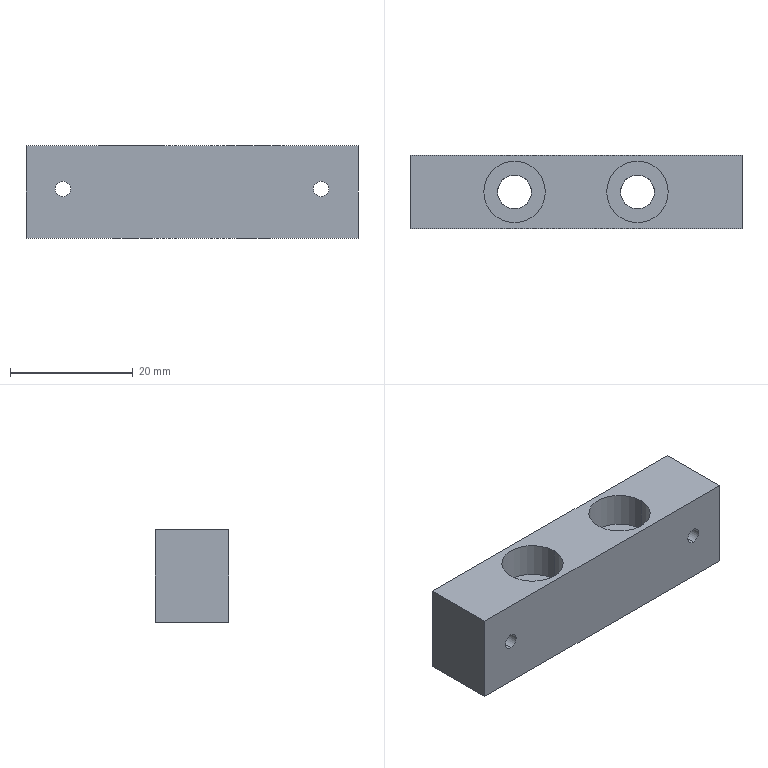Part | STEP file | PN_0024 Mount electronic clip spring mounting plate | 1 solid | 20 faces | box 54 x 12 x 15 mm | volume 8265 mm3 | cylinder 12 | plane 8 | commonest cylinder face diameters 2.5 x4 5.5 x4 10 x4